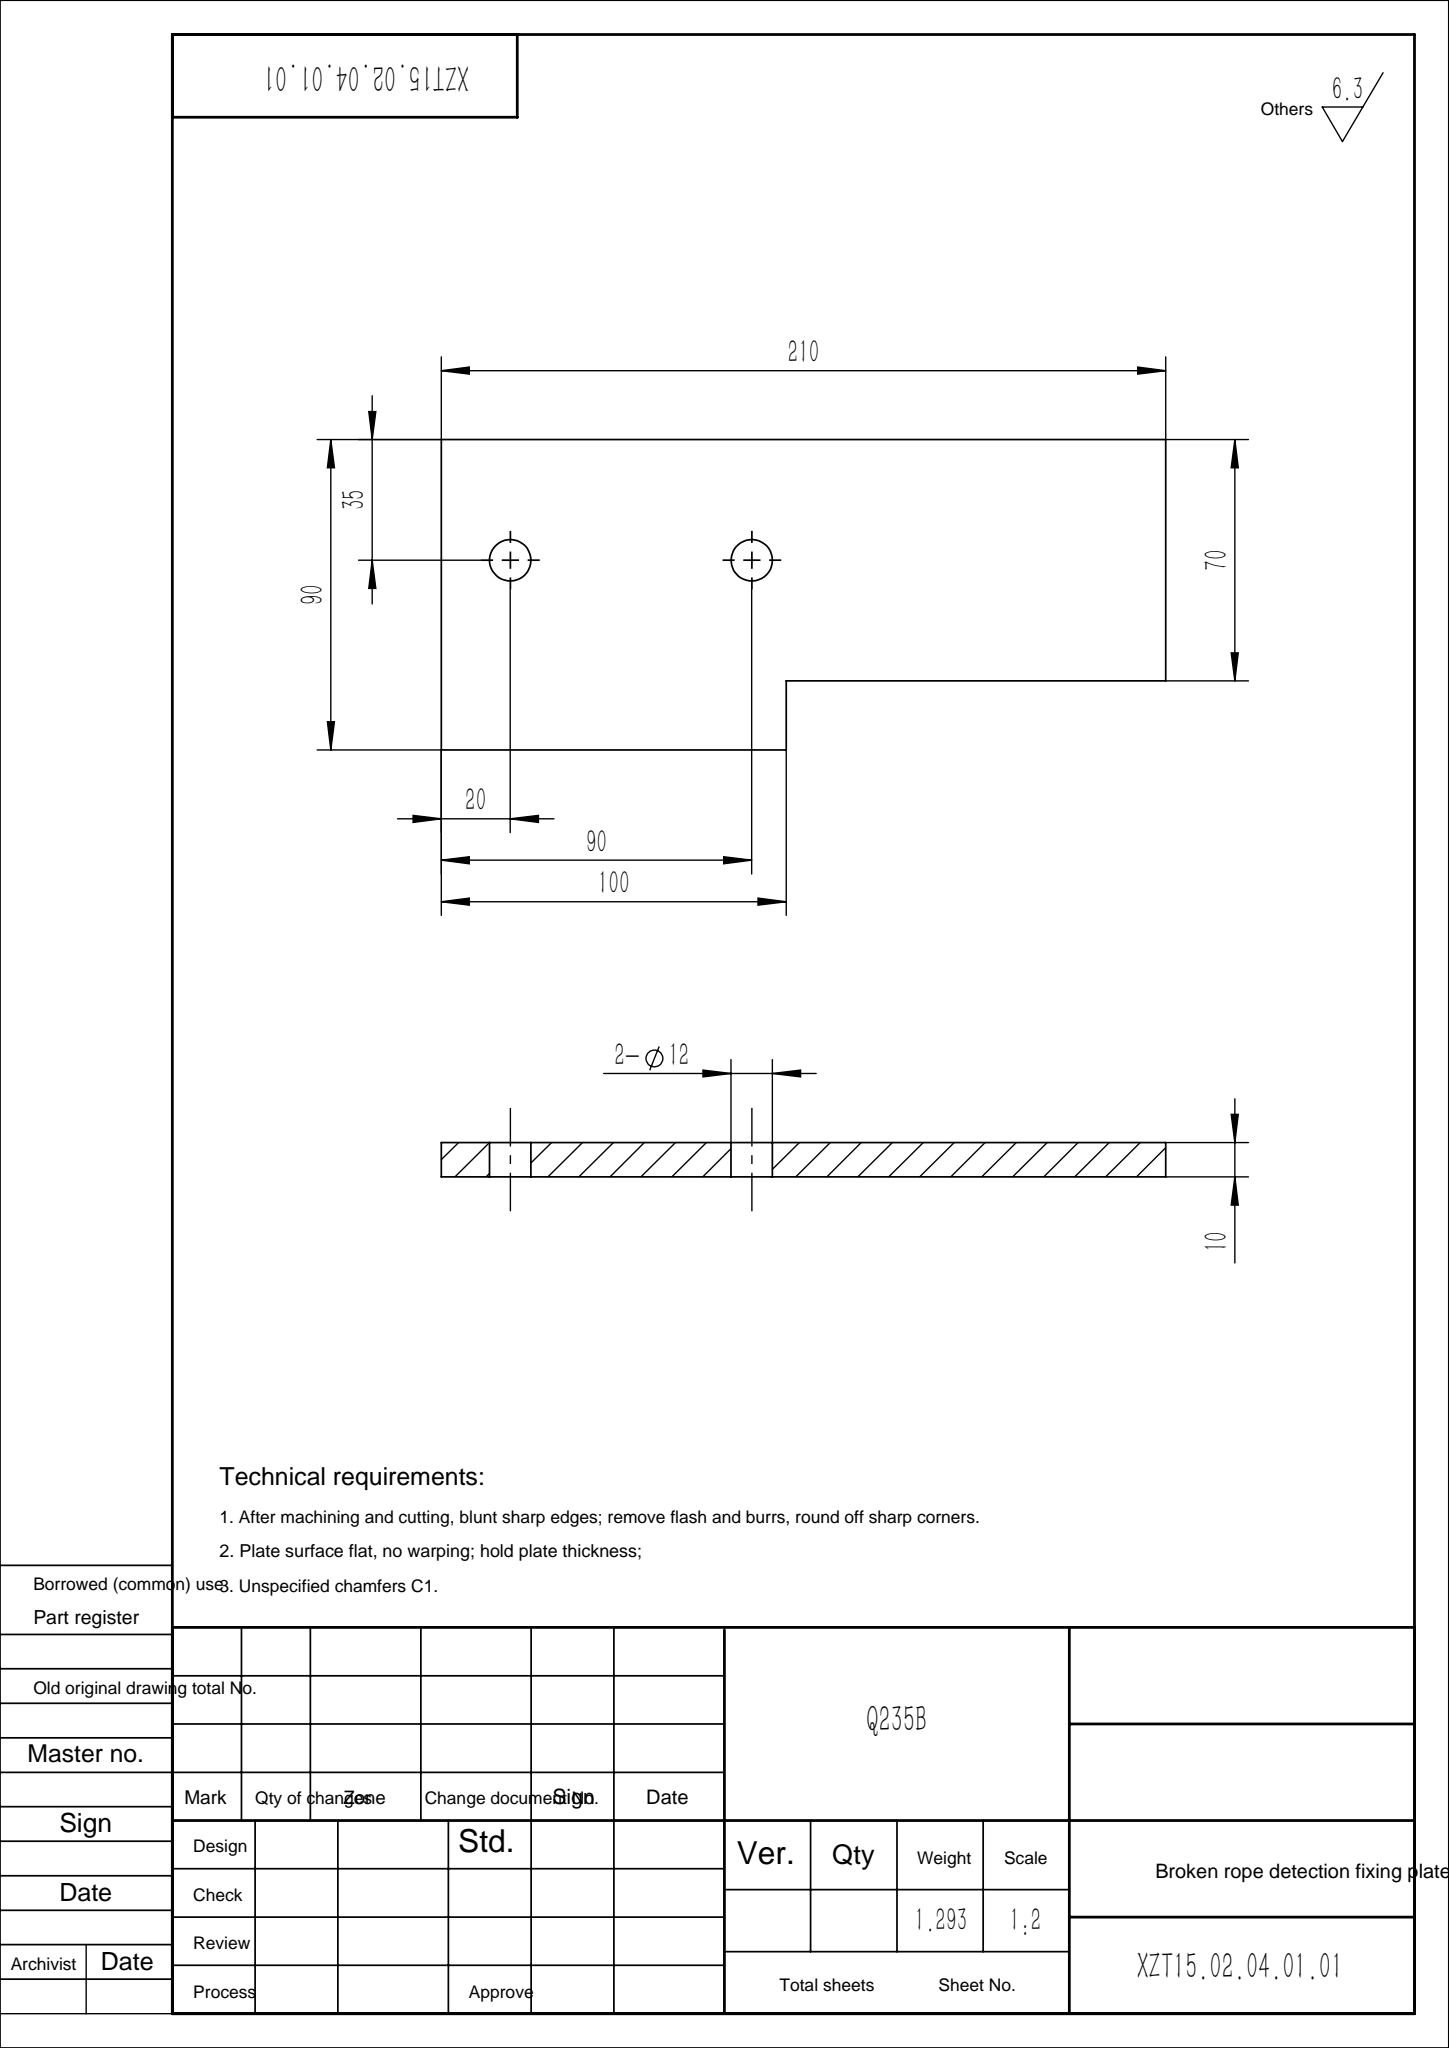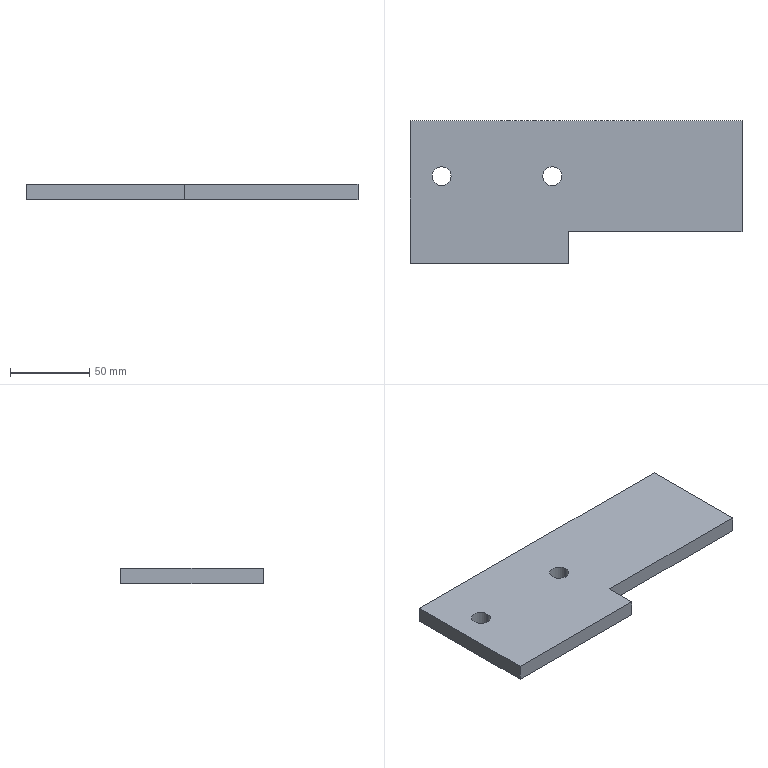Part | SolidWorks | features Extrusion 1, HoleWzd 1 | 1 solid | 12 faces | box 210 x 90 x 10 mm | volume 164738 mm3 | plane 8 | cylinder 4 | commonest cylinder face diameters 12 x4
STEP:
#1=CARTESIAN_POINT('',(26.,55.,-5.));
#2=VERTEX_POINT('',#1);
#3=CARTESIAN_POINT('',(14.,55.,-5.));
#4=VERTEX_POINT('',#3);
#5=CARTESIAN_POINT('',(20.,55.,-5.));
#6=DIRECTION('',(0.,0.,-1.));
#7=DIRECTION('',(-1.,0.,0.));
#8=AXIS2_PLACEMENT_3D('',#5,#6,#7);
#9=CIRCLE('',#8,6.);
#10=EDGE_CURVE('',#2,#4,#9,.T.);
#11=ORIENTED_EDGE('',*,*,#10,.T.);
#12=CARTESIAN_POINT('',(14.,55.,5.));
#13=VERTEX_POINT('',#12);
#14=CARTESIAN_POINT('',(14.,55.,5.));
#15=DIRECTION('',(0.,0.,1.));
#16=VECTOR('',#15,1000.);
#17=LINE('',#14,#16);
#18=EDGE_CURVE('',#4,#13,#17,.T.);
#19=ORIENTED_EDGE('',*,*,#18,.T.);
#20=CARTESIAN_POINT('',(26.,55.,5.));
#21=VERTEX_POINT('',#20);
#22=CARTESIAN_POINT('',(20.,55.,5.));
#23=DIRECTION('',(0.,0.,1.));
#24=DIRECTION('',(1.,0.,0.));
#25=AXIS2_PLACEMENT_3D('',#22,#23,#24);
#26=CIRCLE('',#25,6.);
#27=EDGE_CURVE('',#13,#21,#26,.T.);
#28=ORIENTED_EDGE('',*,*,#27,.T.);
#29=CARTESIAN_POINT('',(26.,55.,5.));
#30=DIRECTION('',(0.,0.,1.));
#31=VECTOR('',#30,1000.);
#32=LINE('',#29,#31);
#33=EDGE_CURVE('',#2,#21,#32,.T.);
#34=ORIENTED_EDGE('',*,*,#33,.F.);
#35=EDGE_LOOP('',(#11,#19,#28,#34));
#36=FACE_OUTER_BOUND('',#35,.T.);
#37=CARTESIAN_POINT('',(20.,55.,5.));
#38=DIRECTION('',(0.,0.,1.));
#39=DIRECTION('',(1.,0.,0.));
#40=AXIS2_PLACEMENT_3D('',#37,#38,#39);
#41=CYLINDRICAL_SURFACE('',#40,6.);
#42=ADVANCED_FACE('',(#36),#41,.F.);
#43=CARTESIAN_POINT('',(96.,55.,-5.));
#44=VERTEX_POINT('',#43);
#45=CARTESIAN_POINT('',(84.,55.,-5.));
#46=VERTEX_POINT('',#45);
#47=CARTESIAN_POINT('',(90.,55.,-5.));
#48=DIRECTION('',(0.,0.,-1.));
#49=DIRECTION('',(-1.,0.,0.));
#50=AXIS2_PLACEMENT_3D('',#47,#48,#49);
#51=CIRCLE('',#50,6.);
#52=EDGE_CURVE('',#44,#46,#51,.T.);
#53=ORIENTED_EDGE('',*,*,#52,.T.);
#54=CARTESIAN_POINT('',(84.,55.,5.));
#55=VERTEX_POINT('',#54);
#56=CARTESIAN_POINT('',(84.,55.,5.));
#57=DIRECTION('',(0.,0.,1.));
#58=VECTOR('',#57,1000.);
#59=LINE('',#56,#58);
#60=EDGE_CURVE('',#46,#55,#59,.T.);
#61=ORIENTED_EDGE('',*,*,#60,.T.);
#62=CARTESIAN_POINT('',(96.,55.,5.));
#63=VERTEX_POINT('',#62);
#64=CARTESIAN_POINT('',(90.,55.,5.));
#65=DIRECTION('',(0.,0.,1.));
#66=DIRECTION('',(1.,0.,0.));
#67=AXIS2_PLACEMENT_3D('',#64,#65,#66);
#68=CIRCLE('',#67,6.);
#69=EDGE_CURVE('',#55,#63,#68,.T.);
#70=ORIENTED_EDGE('',*,*,#69,.T.);
#71=CARTESIAN_POINT('',(96.,55.,5.));
#72=DIRECTION('',(0.,0.,1.));
#73=VECTOR('',#72,1000.);
#74=LINE('',#71,#73);
#75=EDGE_CURVE('',#44,#63,#74,.T.);
#76=ORIENTED_EDGE('',*,*,#75,.F.);
#77=EDGE_LOOP('',(#53,#61,#70,#76));
#78=FACE_OUTER_BOUND('',#77,.T.);
#79=CARTESIAN_POINT('',(90.,55.,5.));
#80=DIRECTION('',(0.,0.,1.));
#81=DIRECTION('',(1.,0.,0.));
#82=AXIS2_PLACEMENT_3D('',#79,#80,#81);
#83=CYLINDRICAL_SURFACE('',#82,6.);
#84=ADVANCED_FACE('',(#78),#83,.F.);
#85=CARTESIAN_POINT('',(0.,0.,-5.));
#86=VERTEX_POINT('',#85);
#87=CARTESIAN_POINT('',(100.,0.,-5.));
#88=VERTEX_POINT('',#87);
#89=CARTESIAN_POINT('',(100.,0.,-5.));
#90=DIRECTION('',(1.,0.,0.));
#91=VECTOR('',#90,1000.);
#92=LINE('',#89,#91);
#93=EDGE_CURVE('',#86,#88,#92,.T.);
#94=ORIENTED_EDGE('',*,*,#93,.T.);
#95=CARTESIAN_POINT('',(100.,0.,5.));
#96=VERTEX_POINT('',#95);
#97=CARTESIAN_POINT('',(100.,0.,5.));
#98=DIRECTION('',(0.,0.,-1.));
#99=VECTOR('',#98,1000.);
#100=LINE('',#97,#99);
#101=EDGE_CURVE('',#96,#88,#100,.T.);
#102=ORIENTED_EDGE('',*,*,#101,.F.);
#103=CARTESIAN_POINT('',(0.,0.,5.));
#104=VERTEX_POINT('',#103);
#105=CARTESIAN_POINT('',(100.,0.,5.));
#106=DIRECTION('',(1.,0.,0.));
#107=VECTOR('',#106,1000.);
#108=LINE('',#105,#107);
#109=EDGE_CURVE('',#104,#96,#108,.T.);
#110=ORIENTED_EDGE('',*,*,#109,.F.);
#111=CARTESIAN_POINT('',(0.,0.,5.));
#112=DIRECTION('',(0.,0.,-1.));
#113=VECTOR('',#112,1000.);
#114=LINE('',#111,#113);
#115=EDGE_CURVE('',#104,#86,#114,.T.);
#116=ORIENTED_EDGE('',*,*,#115,.T.);
#117=EDGE_LOOP('',(#94,#102,#110,#116));
#118=FACE_OUTER_BOUND('',#117,.T.);
#119=CARTESIAN_POINT('',(100.,0.,5.));
#120=DIRECTION('',(0.,1.,0.));
#121=DIRECTION('',(0.,0.,1.));
#122=AXIS2_PLACEMENT_3D('',#119,#120,#121);
#123=PLANE('',#122);
#124=ADVANCED_FACE('',(#118),#123,.F.);
#125=CARTESIAN_POINT('',(100.,20.,-5.));
#126=VERTEX_POINT('',#125);
#127=CARTESIAN_POINT('',(100.,20.,-5.));
#128=DIRECTION('',(0.,1.,0.));
#129=VECTOR('',#128,1000.);
#130=LINE('',#127,#129);
#131=EDGE_CURVE('',#88,#126,#130,.T.);
#132=ORIENTED_EDGE('',*,*,#131,.T.);
#133=CARTESIAN_POINT('',(100.,20.,5.));
#134=VERTEX_POINT('',#133);
#135=CARTESIAN_POINT('',(100.,20.,5.));
#136=DIRECTION('',(0.,0.,-1.));
#137=VECTOR('',#136,1000.);
#138=LINE('',#135,#137);
#139=EDGE_CURVE('',#134,#126,#138,.T.);
#140=ORIENTED_EDGE('',*,*,#139,.F.);
#141=CARTESIAN_POINT('',(100.,20.,5.));
#142=DIRECTION('',(0.,1.,0.));
#143=VECTOR('',#142,1000.);
#144=LINE('',#141,#143);
#145=EDGE_CURVE('',#96,#134,#144,.T.);
#146=ORIENTED_EDGE('',*,*,#145,.F.);
#147=ORIENTED_EDGE('',*,*,#101,.T.);
#148=EDGE_LOOP('',(#132,#140,#146,#147));
#149=FACE_OUTER_BOUND('',#148,.T.);
#150=CARTESIAN_POINT('',(100.,20.,5.));
#151=DIRECTION('',(-1.,0.,0.));
#152=DIRECTION('',(0.,0.,1.));
#153=AXIS2_PLACEMENT_3D('',#150,#151,#152);
#154=PLANE('',#153);
#155=ADVANCED_FACE('',(#149),#154,.F.);
#156=CARTESIAN_POINT('',(210.,20.,-5.));
#157=VERTEX_POINT('',#156);
#158=CARTESIAN_POINT('',(210.,20.,-5.));
#159=DIRECTION('',(1.,0.,0.));
#160=VECTOR('',#159,1000.);
#161=LINE('',#158,#160);
#162=EDGE_CURVE('',#126,#157,#161,.T.);
#163=ORIENTED_EDGE('',*,*,#162,.T.);
#164=CARTESIAN_POINT('',(210.,20.,5.));
#165=VERTEX_POINT('',#164);
#166=CARTESIAN_POINT('',(210.,20.,5.));
#167=DIRECTION('',(0.,0.,-1.));
#168=VECTOR('',#167,1000.);
#169=LINE('',#166,#168);
#170=EDGE_CURVE('',#165,#157,#169,.T.);
#171=ORIENTED_EDGE('',*,*,#170,.F.);
#172=CARTESIAN_POINT('',(210.,20.,5.));
#173=DIRECTION('',(1.,0.,0.));
#174=VECTOR('',#173,1000.);
#175=LINE('',#172,#174);
#176=EDGE_CURVE('',#134,#165,#175,.T.);
#177=ORIENTED_EDGE('',*,*,#176,.F.);
#178=ORIENTED_EDGE('',*,*,#139,.T.);
#179=EDGE_LOOP('',(#163,#171,#177,#178));
#180=FACE_OUTER_BOUND('',#179,.T.);
#181=CARTESIAN_POINT('',(210.,20.,5.));
#182=DIRECTION('',(0.,1.,0.));
#183=DIRECTION('',(-1.,0.,0.));
#184=AXIS2_PLACEMENT_3D('',#181,#182,#183);
#185=PLANE('',#184);
#186=ADVANCED_FACE('',(#180),#185,.F.);
#187=CARTESIAN_POINT('',(210.,90.,-5.));
#188=VERTEX_POINT('',#187);
#189=CARTESIAN_POINT('',(210.,90.,-5.));
#190=DIRECTION('',(0.,1.,0.));
#191=VECTOR('',#190,1000.);
#192=LINE('',#189,#191);
#193=EDGE_CURVE('',#157,#188,#192,.T.);
#194=ORIENTED_EDGE('',*,*,#193,.T.);
#195=CARTESIAN_POINT('',(210.,90.,5.));
#196=VERTEX_POINT('',#195);
#197=CARTESIAN_POINT('',(210.,90.,5.));
#198=DIRECTION('',(0.,0.,-1.));
#199=VECTOR('',#198,1000.);
#200=LINE('',#197,#199);
#201=EDGE_CURVE('',#196,#188,#200,.T.);
#202=ORIENTED_EDGE('',*,*,#201,.F.);
#203=CARTESIAN_POINT('',(210.,90.,5.));
#204=DIRECTION('',(0.,1.,0.));
#205=VECTOR('',#204,1000.);
#206=LINE('',#203,#205);
#207=EDGE_CURVE('',#165,#196,#206,.T.);
#208=ORIENTED_EDGE('',*,*,#207,.F.);
#209=ORIENTED_EDGE('',*,*,#170,.T.);
#210=EDGE_LOOP('',(#194,#202,#208,#209));
#211=FACE_OUTER_BOUND('',#210,.T.);
#212=CARTESIAN_POINT('',(210.,90.,5.));
#213=DIRECTION('',(-1.,0.,0.));
#214=DIRECTION('',(0.,-1.,0.));
#215=AXIS2_PLACEMENT_3D('',#212,#213,#214);
#216=PLANE('',#215);
#217=ADVANCED_FACE('',(#211),#216,.F.);
#218=CARTESIAN_POINT('',(0.,90.,-5.));
#219=VERTEX_POINT('',#218);
#220=CARTESIAN_POINT('',(0.,90.,-5.));
#221=DIRECTION('',(-1.,0.,0.));
#222=VECTOR('',#221,1000.);
#223=LINE('',#220,#222);
#224=EDGE_CURVE('',#188,#219,#223,.T.);
#225=ORIENTED_EDGE('',*,*,#224,.T.);
#226=CARTESIAN_POINT('',(0.,90.,5.));
#227=VERTEX_POINT('',#226);
#228=CARTESIAN_POINT('',(0.,90.,5.));
#229=DIRECTION('',(0.,0.,-1.));
#230=VECTOR('',#229,1000.);
#231=LINE('',#228,#230);
#232=EDGE_CURVE('',#227,#219,#231,.T.);
#233=ORIENTED_EDGE('',*,*,#232,.F.);
#234=CARTESIAN_POINT('',(0.,90.,5.));
#235=DIRECTION('',(-1.,0.,0.));
#236=VECTOR('',#235,1000.);
#237=LINE('',#234,#236);
#238=EDGE_CURVE('',#196,#227,#237,.T.);
#239=ORIENTED_EDGE('',*,*,#238,.F.);
#240=ORIENTED_EDGE('',*,*,#201,.T.);
#241=EDGE_LOOP('',(#225,#233,#239,#240));
#242=FACE_OUTER_BOUND('',#241,.T.);
#243=CARTESIAN_POINT('',(0.,90.,5.));
#244=DIRECTION('',(0.,-1.,0.));
#245=DIRECTION('',(0.,0.,-1.));
#246=AXIS2_PLACEMENT_3D('',#243,#244,#245);
#247=PLANE('',#246);
#248=ADVANCED_FACE('',(#242),#247,.F.);
#249=CARTESIAN_POINT('',(0.,0.,-5.));
#250=DIRECTION('',(0.,-1.,0.));
#251=VECTOR('',#250,1000.);
#252=LINE('',#249,#251);
#253=EDGE_CURVE('',#219,#86,#252,.T.);
#254=ORIENTED_EDGE('',*,*,#253,.T.);
#255=ORIENTED_EDGE('',*,*,#115,.F.);
#256=CARTESIAN_POINT('',(0.,0.,5.));
#257=DIRECTION('',(0.,-1.,0.));
#258=VECTOR('',#257,1000.);
#259=LINE('',#256,#258);
#260=EDGE_CURVE('',#227,#104,#259,.T.);
#261=ORIENTED_EDGE('',*,*,#260,.F.);
#262=ORIENTED_EDGE('',*,*,#232,.T.);
#263=EDGE_LOOP('',(#254,#255,#261,#262));
#264=FACE_OUTER_BOUND('',#263,.T.);
#265=CARTESIAN_POINT('',(0.,0.,5.));
#266=DIRECTION('',(1.,0.,0.));
#267=DIRECTION('',(0.,0.,-1.));
#268=AXIS2_PLACEMENT_3D('',#265,#266,#267);
#269=PLANE('',#268);
#270=ADVANCED_FACE('',(#264),#269,.F.);
#271=CARTESIAN_POINT('',(20.,55.,5.));
#272=DIRECTION('',(0.,0.,1.));
#273=DIRECTION('',(1.,0.,0.));
#274=AXIS2_PLACEMENT_3D('',#271,#272,#273);
#275=CIRCLE('',#274,6.);
#276=EDGE_CURVE('',#21,#13,#275,.T.);
#277=ORIENTED_EDGE('',*,*,#276,.F.);
#278=ORIENTED_EDGE('',*,*,#27,.F.);
#279=EDGE_LOOP('',(#277,#278));
#280=FACE_BOUND('',#279,.T.);
#281=CARTESIAN_POINT('',(90.,55.,5.));
#282=DIRECTION('',(0.,0.,1.));
#283=DIRECTION('',(1.,0.,0.));
#284=AXIS2_PLACEMENT_3D('',#281,#282,#283);
#285=CIRCLE('',#284,6.);
#286=EDGE_CURVE('',#63,#55,#285,.T.);
#287=ORIENTED_EDGE('',*,*,#286,.F.);
#288=ORIENTED_EDGE('',*,*,#69,.F.);
#289=EDGE_LOOP('',(#287,#288));
#290=FACE_BOUND('',#289,.T.);
#291=ORIENTED_EDGE('',*,*,#109,.T.);
#292=ORIENTED_EDGE('',*,*,#145,.T.);
#293=ORIENTED_EDGE('',*,*,#176,.T.);
#294=ORIENTED_EDGE('',*,*,#207,.T.);
#295=ORIENTED_EDGE('',*,*,#238,.T.);
#296=ORIENTED_EDGE('',*,*,#260,.T.);
#297=EDGE_LOOP('',(#291,#292,#293,#294,#295,#296));
#298=FACE_OUTER_BOUND('',#297,.T.);
#299=CARTESIAN_POINT('',(0.,0.,5.));
#300=DIRECTION('',(0.,0.,-1.));
#301=DIRECTION('',(-1.,0.,0.));
#302=AXIS2_PLACEMENT_3D('',#299,#300,#301);
#303=PLANE('',#302);
#304=ADVANCED_FACE('',(#280,#290,#298),#303,.F.);
#305=ORIENTED_EDGE('',*,*,#10,.F.);
#306=CARTESIAN_POINT('',(20.,55.,-5.));
#307=DIRECTION('',(0.,0.,-1.));
#308=DIRECTION('',(-1.,0.,0.));
#309=AXIS2_PLACEMENT_3D('',#306,#307,#308);
#310=CIRCLE('',#309,6.);
#311=EDGE_CURVE('',#4,#2,#310,.T.);
#312=ORIENTED_EDGE('',*,*,#311,.F.);
#313=EDGE_LOOP('',(#305,#312));
#314=FACE_BOUND('',#313,.T.);
#315=ORIENTED_EDGE('',*,*,#52,.F.);
#316=CARTESIAN_POINT('',(90.,55.,-5.));
#317=DIRECTION('',(0.,0.,-1.));
#318=DIRECTION('',(-1.,0.,0.));
#319=AXIS2_PLACEMENT_3D('',#316,#317,#318);
#320=CIRCLE('',#319,6.);
#321=EDGE_CURVE('',#46,#44,#320,.T.);
#322=ORIENTED_EDGE('',*,*,#321,.F.);
#323=EDGE_LOOP('',(#315,#322));
#324=FACE_BOUND('',#323,.T.);
#325=ORIENTED_EDGE('',*,*,#93,.F.);
#326=ORIENTED_EDGE('',*,*,#253,.F.);
#327=ORIENTED_EDGE('',*,*,#224,.F.);
#328=ORIENTED_EDGE('',*,*,#193,.F.);
#329=ORIENTED_EDGE('',*,*,#162,.F.);
#330=ORIENTED_EDGE('',*,*,#131,.F.);
#331=EDGE_LOOP('',(#325,#326,#327,#328,#329,#330));
#332=FACE_OUTER_BOUND('',#331,.T.);
#333=CARTESIAN_POINT('',(0.,0.,-5.));
#334=DIRECTION('',(0.,0.,-1.));
#335=DIRECTION('',(-1.,0.,0.));
#336=AXIS2_PLACEMENT_3D('',#333,#334,#335);
#337=PLANE('',#336);
#338=ADVANCED_FACE('',(#314,#324,#332),#337,.T.);
#339=ORIENTED_EDGE('',*,*,#60,.F.);
#340=ORIENTED_EDGE('',*,*,#321,.T.);
#341=ORIENTED_EDGE('',*,*,#75,.T.);
#342=ORIENTED_EDGE('',*,*,#286,.T.);
#343=EDGE_LOOP('',(#339,#340,#341,#342));
#344=FACE_OUTER_BOUND('',#343,.T.);
#345=CARTESIAN_POINT('',(90.,55.,5.));
#346=DIRECTION('',(0.,0.,1.));
#347=DIRECTION('',(1.,0.,0.));
#348=AXIS2_PLACEMENT_3D('',#345,#346,#347);
#349=CYLINDRICAL_SURFACE('',#348,6.);
#350=ADVANCED_FACE('',(#344),#349,.F.);
#351=ORIENTED_EDGE('',*,*,#18,.F.);
#352=ORIENTED_EDGE('',*,*,#311,.T.);
#353=ORIENTED_EDGE('',*,*,#33,.T.);
#354=ORIENTED_EDGE('',*,*,#276,.T.);
#355=EDGE_LOOP('',(#351,#352,#353,#354));
#356=FACE_OUTER_BOUND('',#355,.T.);
#357=CARTESIAN_POINT('',(20.,55.,5.));
#358=DIRECTION('',(0.,0.,1.));
#359=DIRECTION('',(1.,0.,0.));
#360=AXIS2_PLACEMENT_3D('',#357,#358,#359);
#361=CYLINDRICAL_SURFACE('',#360,6.);
#362=ADVANCED_FACE('',(#356),#361,.F.);
#363=CLOSED_SHELL('',(#42,#84,#124,#155,#186,#217,#248,#270,#304,#338,#350,#362));
#364=MANIFOLD_SOLID_BREP('',#363);
#365=CARTESIAN_POINT('',(0.,0.,0.));
#366=DIRECTION('',(0.,0.,1.));
#367=DIRECTION('',(1.,0.,0.));
#368=AXIS2_PLACEMENT_3D('',#365,#366,#367);
#369=(LENGTH_UNIT()NAMED_UNIT(*)SI_UNIT(.MILLI.,.METRE.));
#370=UNCERTAINTY_MEASURE_WITH_UNIT(LENGTH_MEASURE(0.00001),#369,'','');
#371=(NAMED_UNIT(*)PLANE_ANGLE_UNIT()SI_UNIT($,.RADIAN.));
#372=(NAMED_UNIT(*)SI_UNIT($,.STERADIAN.)SOLID_ANGLE_UNIT());
#373=(GEOMETRIC_REPRESENTATION_CONTEXT(3)GLOBAL_UNCERTAINTY_ASSIGNED_CONTEXT((#370))GLOBAL_UNIT_ASSIGNED_CONTEXT((#369,#371,#372))REPRESENTATION_CONTEXT('',''));
#374=ADVANCED_BREP_SHAPE_REPRESENTATION('',(#364,#368),#373);